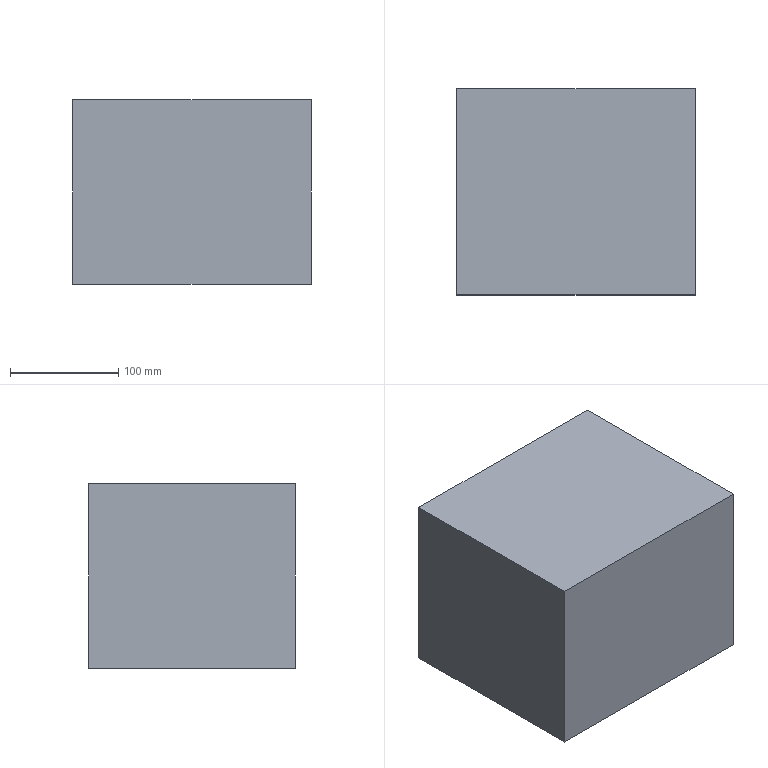Part | STEP file | SceondREWTRT_Default | 1 solid | 6 faces | box 220 x 190 x 170 mm | volume 7106000 mm3 | plane 6
STEP:
#1=CARTESIAN_POINT('',(0.,0.,0.));
#2=DIRECTION('',(0.,0.,1.));
#3=DIRECTION('',(1.,0.,0.));
#4=AXIS2_PLACEMENT_3D('',#1,#2,#3);
#5=CARTESIAN_POINT('',(-110.,0.,-85.));
#6=VERTEX_POINT('',#5);
#7=CARTESIAN_POINT('',(-110.,0.,85.));
#8=VERTEX_POINT('',#7);
#9=CARTESIAN_POINT('',(-110.,0.,85.));
#10=DIRECTION('',(0.,0.,1.));
#11=VECTOR('',#10,1.);
#12=LINE('',#9,#11);
#13=CARTESIAN_POINT('',(-110.,190.,85.));
#14=DIRECTION('',(1.,0.,0.));
#15=DIRECTION('',(0.,0.,-1.));
#16=AXIS2_PLACEMENT_3D('',#13,#14,#15);
#17=PLANE('',#16);
#18=CARTESIAN_POINT('',(0.,-190.));
#19=DIRECTION('',(-1.,0.));
#20=VECTOR('',#19,1.);
#21=LINE('',#18,#20);
#22=(GEOMETRIC_REPRESENTATION_CONTEXT(2)PARAMETRIC_REPRESENTATION_CONTEXT()REPRESENTATION_CONTEXT('',''));
#23=DEFINITIONAL_REPRESENTATION('',(#21),#22);
#24=PCURVE('',#17,#23);
#25=CARTESIAN_POINT('',(0.,0.,0.));
#26=DIRECTION('',(0.,1.,0.));
#27=DIRECTION('',(0.,0.,1.));
#28=AXIS2_PLACEMENT_3D('',#25,#26,#27);
#29=PLANE('',#28);
#30=CARTESIAN_POINT('',(85.,-110.));
#31=DIRECTION('',(1.,0.));
#32=VECTOR('',#31,1.);
#33=LINE('',#30,#32);
#34=(GEOMETRIC_REPRESENTATION_CONTEXT(2)PARAMETRIC_REPRESENTATION_CONTEXT()REPRESENTATION_CONTEXT('',''));
#35=DEFINITIONAL_REPRESENTATION('',(#33),#34);
#36=PCURVE('',#29,#35);
#37=SURFACE_CURVE('',#12,(#24,#36),.PCURVE_S1.);
#38=EDGE_CURVE('',#6,#8,#37,.T.);
#39=ORIENTED_EDGE('',*,*,#38,.T.);
#40=CARTESIAN_POINT('',(-110.,190.,85.));
#41=VERTEX_POINT('',#40);
#42=CARTESIAN_POINT('',(-110.,190.,85.));
#43=DIRECTION('',(0.,-1.,0.));
#44=VECTOR('',#43,1.);
#45=LINE('',#42,#44);
#46=CARTESIAN_POINT('',(0.,0.));
#47=DIRECTION('',(0.,-1.));
#48=VECTOR('',#47,1.);
#49=LINE('',#46,#48);
#50=(GEOMETRIC_REPRESENTATION_CONTEXT(2)PARAMETRIC_REPRESENTATION_CONTEXT()REPRESENTATION_CONTEXT('',''));
#51=DEFINITIONAL_REPRESENTATION('',(#49),#50);
#52=PCURVE('',#17,#51);
#53=CARTESIAN_POINT('',(110.,190.,85.));
#54=DIRECTION('',(0.,0.,-1.));
#55=DIRECTION('',(-1.,0.,0.));
#56=AXIS2_PLACEMENT_3D('',#53,#54,#55);
#57=PLANE('',#56);
#58=CARTESIAN_POINT('',(220.,0.));
#59=DIRECTION('',(0.,-1.));
#60=VECTOR('',#59,1.);
#61=LINE('',#58,#60);
#62=(GEOMETRIC_REPRESENTATION_CONTEXT(2)PARAMETRIC_REPRESENTATION_CONTEXT()REPRESENTATION_CONTEXT('',''));
#63=DEFINITIONAL_REPRESENTATION('',(#61),#62);
#64=PCURVE('',#57,#63);
#65=SURFACE_CURVE('',#45,(#52,#64),.PCURVE_S1.);
#66=EDGE_CURVE('',#41,#8,#65,.T.);
#67=ORIENTED_EDGE('',*,*,#66,.F.);
#68=CARTESIAN_POINT('',(-110.,190.,-85.));
#69=VERTEX_POINT('',#68);
#70=CARTESIAN_POINT('',(-110.,190.,85.));
#71=DIRECTION('',(0.,0.,1.));
#72=VECTOR('',#71,1.);
#73=LINE('',#70,#72);
#74=CARTESIAN_POINT('',(0.,0.));
#75=DIRECTION('',(-1.,0.));
#76=VECTOR('',#75,1.);
#77=LINE('',#74,#76);
#78=(GEOMETRIC_REPRESENTATION_CONTEXT(2)PARAMETRIC_REPRESENTATION_CONTEXT()REPRESENTATION_CONTEXT('',''));
#79=DEFINITIONAL_REPRESENTATION('',(#77),#78);
#80=PCURVE('',#17,#79);
#81=CARTESIAN_POINT('',(0.,190.,0.));
#82=DIRECTION('',(0.,1.,0.));
#83=DIRECTION('',(0.,0.,1.));
#84=AXIS2_PLACEMENT_3D('',#81,#82,#83);
#85=PLANE('',#84);
#86=CARTESIAN_POINT('',(85.,-110.));
#87=DIRECTION('',(1.,0.));
#88=VECTOR('',#87,1.);
#89=LINE('',#86,#88);
#90=(GEOMETRIC_REPRESENTATION_CONTEXT(2)PARAMETRIC_REPRESENTATION_CONTEXT()REPRESENTATION_CONTEXT('',''));
#91=DEFINITIONAL_REPRESENTATION('',(#89),#90);
#92=PCURVE('',#85,#91);
#93=SURFACE_CURVE('',#73,(#80,#92),.PCURVE_S1.);
#94=EDGE_CURVE('',#69,#41,#93,.T.);
#95=ORIENTED_EDGE('',*,*,#94,.F.);
#96=CARTESIAN_POINT('',(-110.,190.,-85.));
#97=DIRECTION('',(0.,-1.,0.));
#98=VECTOR('',#97,1.);
#99=LINE('',#96,#98);
#100=CARTESIAN_POINT('',(170.,0.));
#101=DIRECTION('',(0.,-1.));
#102=VECTOR('',#101,1.);
#103=LINE('',#100,#102);
#104=(GEOMETRIC_REPRESENTATION_CONTEXT(2)PARAMETRIC_REPRESENTATION_CONTEXT()REPRESENTATION_CONTEXT('',''));
#105=DEFINITIONAL_REPRESENTATION('',(#103),#104);
#106=PCURVE('',#17,#105);
#107=CARTESIAN_POINT('',(110.,190.,-85.));
#108=DIRECTION('',(0.,0.,1.));
#109=DIRECTION('',(1.,0.,0.));
#110=AXIS2_PLACEMENT_3D('',#107,#108,#109);
#111=PLANE('',#110);
#112=CARTESIAN_POINT('',(-220.,0.));
#113=DIRECTION('',(0.,-1.));
#114=VECTOR('',#113,1.);
#115=LINE('',#112,#114);
#116=(GEOMETRIC_REPRESENTATION_CONTEXT(2)PARAMETRIC_REPRESENTATION_CONTEXT()REPRESENTATION_CONTEXT('',''));
#117=DEFINITIONAL_REPRESENTATION('',(#115),#116);
#118=PCURVE('',#111,#117);
#119=SURFACE_CURVE('',#99,(#106,#118),.PCURVE_S1.);
#120=EDGE_CURVE('',#69,#6,#119,.T.);
#121=ORIENTED_EDGE('',*,*,#120,.T.);
#122=EDGE_LOOP('',(#39,#67,#95,#121));
#123=FACE_BOUND('',#122,.T.);
#124=ADVANCED_FACE('',(#123),#17,.F.);
#125=CARTESIAN_POINT('',(110.,0.,85.));
#126=VERTEX_POINT('',#125);
#127=CARTESIAN_POINT('',(110.,0.,85.));
#128=DIRECTION('',(1.,0.,0.));
#129=VECTOR('',#128,1.);
#130=LINE('',#127,#129);
#131=CARTESIAN_POINT('',(0.,-190.));
#132=DIRECTION('',(-1.,0.));
#133=VECTOR('',#132,1.);
#134=LINE('',#131,#133);
#135=(GEOMETRIC_REPRESENTATION_CONTEXT(2)PARAMETRIC_REPRESENTATION_CONTEXT()REPRESENTATION_CONTEXT('',''));
#136=DEFINITIONAL_REPRESENTATION('',(#134),#135);
#137=PCURVE('',#57,#136);
#138=CARTESIAN_POINT('',(85.,110.));
#139=DIRECTION('',(0.,1.));
#140=VECTOR('',#139,1.);
#141=LINE('',#138,#140);
#142=(GEOMETRIC_REPRESENTATION_CONTEXT(2)PARAMETRIC_REPRESENTATION_CONTEXT()REPRESENTATION_CONTEXT('',''));
#143=DEFINITIONAL_REPRESENTATION('',(#141),#142);
#144=PCURVE('',#29,#143);
#145=SURFACE_CURVE('',#130,(#137,#144),.PCURVE_S1.);
#146=EDGE_CURVE('',#8,#126,#145,.T.);
#147=ORIENTED_EDGE('',*,*,#146,.T.);
#148=CARTESIAN_POINT('',(110.,190.,85.));
#149=VERTEX_POINT('',#148);
#150=CARTESIAN_POINT('',(110.,190.,85.));
#151=DIRECTION('',(0.,-1.,0.));
#152=VECTOR('',#151,1.);
#153=LINE('',#150,#152);
#154=CARTESIAN_POINT('',(0.,0.));
#155=DIRECTION('',(0.,-1.));
#156=VECTOR('',#155,1.);
#157=LINE('',#154,#156);
#158=(GEOMETRIC_REPRESENTATION_CONTEXT(2)PARAMETRIC_REPRESENTATION_CONTEXT()REPRESENTATION_CONTEXT('',''));
#159=DEFINITIONAL_REPRESENTATION('',(#157),#158);
#160=PCURVE('',#57,#159);
#161=CARTESIAN_POINT('',(110.,190.,85.));
#162=DIRECTION('',(-1.,0.,0.));
#163=DIRECTION('',(0.,0.,1.));
#164=AXIS2_PLACEMENT_3D('',#161,#162,#163);
#165=PLANE('',#164);
#166=CARTESIAN_POINT('',(0.,0.));
#167=DIRECTION('',(0.,-1.));
#168=VECTOR('',#167,1.);
#169=LINE('',#166,#168);
#170=(GEOMETRIC_REPRESENTATION_CONTEXT(2)PARAMETRIC_REPRESENTATION_CONTEXT()REPRESENTATION_CONTEXT('',''));
#171=DEFINITIONAL_REPRESENTATION('',(#169),#170);
#172=PCURVE('',#165,#171);
#173=SURFACE_CURVE('',#153,(#160,#172),.PCURVE_S1.);
#174=EDGE_CURVE('',#149,#126,#173,.T.);
#175=ORIENTED_EDGE('',*,*,#174,.F.);
#176=CARTESIAN_POINT('',(110.,190.,85.));
#177=DIRECTION('',(1.,0.,0.));
#178=VECTOR('',#177,1.);
#179=LINE('',#176,#178);
#180=CARTESIAN_POINT('',(0.,0.));
#181=DIRECTION('',(-1.,0.));
#182=VECTOR('',#181,1.);
#183=LINE('',#180,#182);
#184=(GEOMETRIC_REPRESENTATION_CONTEXT(2)PARAMETRIC_REPRESENTATION_CONTEXT()REPRESENTATION_CONTEXT('',''));
#185=DEFINITIONAL_REPRESENTATION('',(#183),#184);
#186=PCURVE('',#57,#185);
#187=CARTESIAN_POINT('',(85.,110.));
#188=DIRECTION('',(0.,1.));
#189=VECTOR('',#188,1.);
#190=LINE('',#187,#189);
#191=(GEOMETRIC_REPRESENTATION_CONTEXT(2)PARAMETRIC_REPRESENTATION_CONTEXT()REPRESENTATION_CONTEXT('',''));
#192=DEFINITIONAL_REPRESENTATION('',(#190),#191);
#193=PCURVE('',#85,#192);
#194=SURFACE_CURVE('',#179,(#186,#193),.PCURVE_S1.);
#195=EDGE_CURVE('',#41,#149,#194,.T.);
#196=ORIENTED_EDGE('',*,*,#195,.F.);
#197=ORIENTED_EDGE('',*,*,#66,.T.);
#198=EDGE_LOOP('',(#147,#175,#196,#197));
#199=FACE_BOUND('',#198,.T.);
#200=ADVANCED_FACE('',(#199),#57,.F.);
#201=CARTESIAN_POINT('',(110.,0.,-85.));
#202=VERTEX_POINT('',#201);
#203=CARTESIAN_POINT('',(110.,0.,85.));
#204=DIRECTION('',(0.,0.,-1.));
#205=VECTOR('',#204,1.);
#206=LINE('',#203,#205);
#207=CARTESIAN_POINT('',(0.,-190.));
#208=DIRECTION('',(-1.,0.));
#209=VECTOR('',#208,1.);
#210=LINE('',#207,#209);
#211=(GEOMETRIC_REPRESENTATION_CONTEXT(2)PARAMETRIC_REPRESENTATION_CONTEXT()REPRESENTATION_CONTEXT('',''));
#212=DEFINITIONAL_REPRESENTATION('',(#210),#211);
#213=PCURVE('',#165,#212);
#214=CARTESIAN_POINT('',(85.,110.));
#215=DIRECTION('',(-1.,0.));
#216=VECTOR('',#215,1.);
#217=LINE('',#214,#216);
#218=(GEOMETRIC_REPRESENTATION_CONTEXT(2)PARAMETRIC_REPRESENTATION_CONTEXT()REPRESENTATION_CONTEXT('',''));
#219=DEFINITIONAL_REPRESENTATION('',(#217),#218);
#220=PCURVE('',#29,#219);
#221=SURFACE_CURVE('',#206,(#213,#220),.PCURVE_S1.);
#222=EDGE_CURVE('',#126,#202,#221,.T.);
#223=ORIENTED_EDGE('',*,*,#222,.T.);
#224=CARTESIAN_POINT('',(110.,190.,-85.));
#225=VERTEX_POINT('',#224);
#226=CARTESIAN_POINT('',(110.,190.,-85.));
#227=DIRECTION('',(0.,-1.,0.));
#228=VECTOR('',#227,1.);
#229=LINE('',#226,#228);
#230=CARTESIAN_POINT('',(-170.,0.));
#231=DIRECTION('',(0.,-1.));
#232=VECTOR('',#231,1.);
#233=LINE('',#230,#232);
#234=(GEOMETRIC_REPRESENTATION_CONTEXT(2)PARAMETRIC_REPRESENTATION_CONTEXT()REPRESENTATION_CONTEXT('',''));
#235=DEFINITIONAL_REPRESENTATION('',(#233),#234);
#236=PCURVE('',#165,#235);
#237=CARTESIAN_POINT('',(0.,0.));
#238=DIRECTION('',(0.,-1.));
#239=VECTOR('',#238,1.);
#240=LINE('',#237,#239);
#241=(GEOMETRIC_REPRESENTATION_CONTEXT(2)PARAMETRIC_REPRESENTATION_CONTEXT()REPRESENTATION_CONTEXT('',''));
#242=DEFINITIONAL_REPRESENTATION('',(#240),#241);
#243=PCURVE('',#111,#242);
#244=SURFACE_CURVE('',#229,(#236,#243),.PCURVE_S1.);
#245=EDGE_CURVE('',#225,#202,#244,.T.);
#246=ORIENTED_EDGE('',*,*,#245,.F.);
#247=CARTESIAN_POINT('',(110.,190.,85.));
#248=DIRECTION('',(0.,0.,-1.));
#249=VECTOR('',#248,1.);
#250=LINE('',#247,#249);
#251=CARTESIAN_POINT('',(0.,0.));
#252=DIRECTION('',(-1.,0.));
#253=VECTOR('',#252,1.);
#254=LINE('',#251,#253);
#255=(GEOMETRIC_REPRESENTATION_CONTEXT(2)PARAMETRIC_REPRESENTATION_CONTEXT()REPRESENTATION_CONTEXT('',''));
#256=DEFINITIONAL_REPRESENTATION('',(#254),#255);
#257=PCURVE('',#165,#256);
#258=CARTESIAN_POINT('',(85.,110.));
#259=DIRECTION('',(-1.,0.));
#260=VECTOR('',#259,1.);
#261=LINE('',#258,#260);
#262=(GEOMETRIC_REPRESENTATION_CONTEXT(2)PARAMETRIC_REPRESENTATION_CONTEXT()REPRESENTATION_CONTEXT('',''));
#263=DEFINITIONAL_REPRESENTATION('',(#261),#262);
#264=PCURVE('',#85,#263);
#265=SURFACE_CURVE('',#250,(#257,#264),.PCURVE_S1.);
#266=EDGE_CURVE('',#149,#225,#265,.T.);
#267=ORIENTED_EDGE('',*,*,#266,.F.);
#268=ORIENTED_EDGE('',*,*,#174,.T.);
#269=EDGE_LOOP('',(#223,#246,#267,#268));
#270=FACE_BOUND('',#269,.T.);
#271=ADVANCED_FACE('',(#270),#165,.F.);
#272=CARTESIAN_POINT('',(110.,0.,-85.));
#273=DIRECTION('',(-1.,0.,0.));
#274=VECTOR('',#273,1.);
#275=LINE('',#272,#274);
#276=CARTESIAN_POINT('',(0.,-190.));
#277=DIRECTION('',(-1.,0.));
#278=VECTOR('',#277,1.);
#279=LINE('',#276,#278);
#280=(GEOMETRIC_REPRESENTATION_CONTEXT(2)PARAMETRIC_REPRESENTATION_CONTEXT()REPRESENTATION_CONTEXT('',''));
#281=DEFINITIONAL_REPRESENTATION('',(#279),#280);
#282=PCURVE('',#111,#281);
#283=CARTESIAN_POINT('',(-85.,110.));
#284=DIRECTION('',(0.,-1.));
#285=VECTOR('',#284,1.);
#286=LINE('',#283,#285);
#287=(GEOMETRIC_REPRESENTATION_CONTEXT(2)PARAMETRIC_REPRESENTATION_CONTEXT()REPRESENTATION_CONTEXT('',''));
#288=DEFINITIONAL_REPRESENTATION('',(#286),#287);
#289=PCURVE('',#29,#288);
#290=SURFACE_CURVE('',#275,(#282,#289),.PCURVE_S1.);
#291=EDGE_CURVE('',#202,#6,#290,.T.);
#292=ORIENTED_EDGE('',*,*,#291,.T.);
#293=ORIENTED_EDGE('',*,*,#120,.F.);
#294=CARTESIAN_POINT('',(110.,190.,-85.));
#295=DIRECTION('',(-1.,0.,0.));
#296=VECTOR('',#295,1.);
#297=LINE('',#294,#296);
#298=CARTESIAN_POINT('',(0.,0.));
#299=DIRECTION('',(-1.,0.));
#300=VECTOR('',#299,1.);
#301=LINE('',#298,#300);
#302=(GEOMETRIC_REPRESENTATION_CONTEXT(2)PARAMETRIC_REPRESENTATION_CONTEXT()REPRESENTATION_CONTEXT('',''));
#303=DEFINITIONAL_REPRESENTATION('',(#301),#302);
#304=PCURVE('',#111,#303);
#305=CARTESIAN_POINT('',(-85.,110.));
#306=DIRECTION('',(0.,-1.));
#307=VECTOR('',#306,1.);
#308=LINE('',#305,#307);
#309=(GEOMETRIC_REPRESENTATION_CONTEXT(2)PARAMETRIC_REPRESENTATION_CONTEXT()REPRESENTATION_CONTEXT('',''));
#310=DEFINITIONAL_REPRESENTATION('',(#308),#309);
#311=PCURVE('',#85,#310);
#312=SURFACE_CURVE('',#297,(#304,#311),.PCURVE_S1.);
#313=EDGE_CURVE('',#225,#69,#312,.T.);
#314=ORIENTED_EDGE('',*,*,#313,.F.);
#315=ORIENTED_EDGE('',*,*,#245,.T.);
#316=EDGE_LOOP('',(#292,#293,#314,#315));
#317=FACE_BOUND('',#316,.T.);
#318=ADVANCED_FACE('',(#317),#111,.F.);
#319=ORIENTED_EDGE('',*,*,#94,.T.);
#320=ORIENTED_EDGE('',*,*,#195,.T.);
#321=ORIENTED_EDGE('',*,*,#266,.T.);
#322=ORIENTED_EDGE('',*,*,#313,.T.);
#323=EDGE_LOOP('',(#319,#320,#321,#322));
#324=FACE_BOUND('',#323,.T.);
#325=ADVANCED_FACE('',(#324),#85,.T.);
#326=ORIENTED_EDGE('',*,*,#38,.F.);
#327=ORIENTED_EDGE('',*,*,#291,.F.);
#328=ORIENTED_EDGE('',*,*,#222,.F.);
#329=ORIENTED_EDGE('',*,*,#146,.F.);
#330=EDGE_LOOP('',(#326,#327,#328,#329));
#331=FACE_BOUND('',#330,.T.);
#332=ADVANCED_FACE('',(#331),#29,.F.);
#333=CLOSED_SHELL('',(#124,#200,#271,#318,#325,#332));
#334=MANIFOLD_SOLID_BREP('',#333);
#335=(LENGTH_UNIT()NAMED_UNIT(*)SI_UNIT(.MILLI.,.METRE.));
#336=UNCERTAINTY_MEASURE_WITH_UNIT(LENGTH_MEASURE(0.0000001),#335,'','');
#337=(NAMED_UNIT(*)PLANE_ANGLE_UNIT()SI_UNIT($,.RADIAN.));
#338=(NAMED_UNIT(*)SI_UNIT($,.STERADIAN.)SOLID_ANGLE_UNIT());
#339=(GEOMETRIC_REPRESENTATION_CONTEXT(3)GLOBAL_UNCERTAINTY_ASSIGNED_CONTEXT((#336))GLOBAL_UNIT_ASSIGNED_CONTEXT((#335,#337,#338))REPRESENTATION_CONTEXT('',''));
#340=ADVANCED_BREP_SHAPE_REPRESENTATION('',(#4,#334),#339);